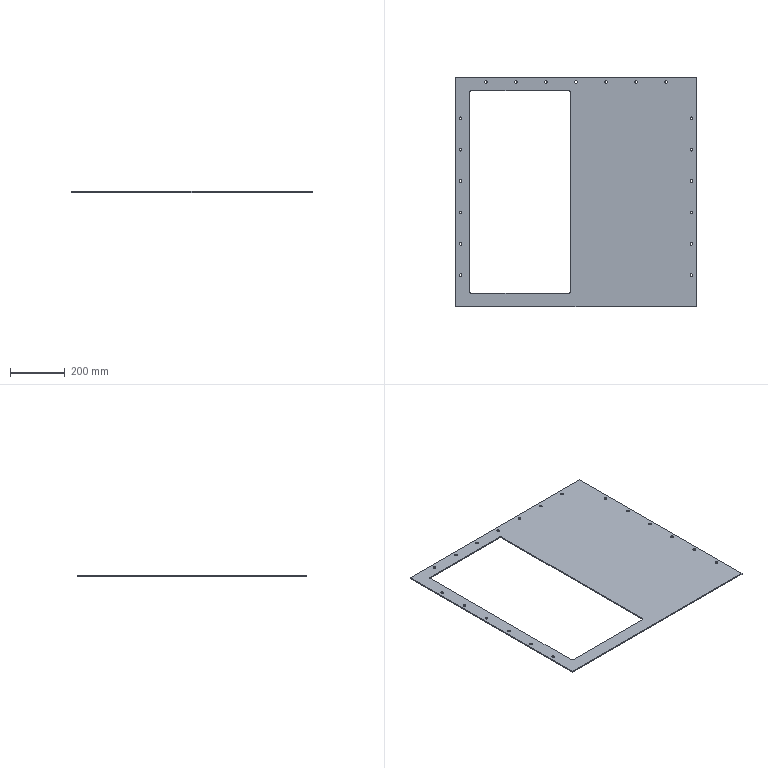Part | SolidWorks | features Fillet 1, FlatPattern 1, SMBaseFlange 1, SheetMetal 1 | 1 solid | 52 faces | box 880 x 840 x 4 mm | volume 1855717 mm3 | cylinder 42 | plane 10 | commonest cylinder face diameters 10 x42